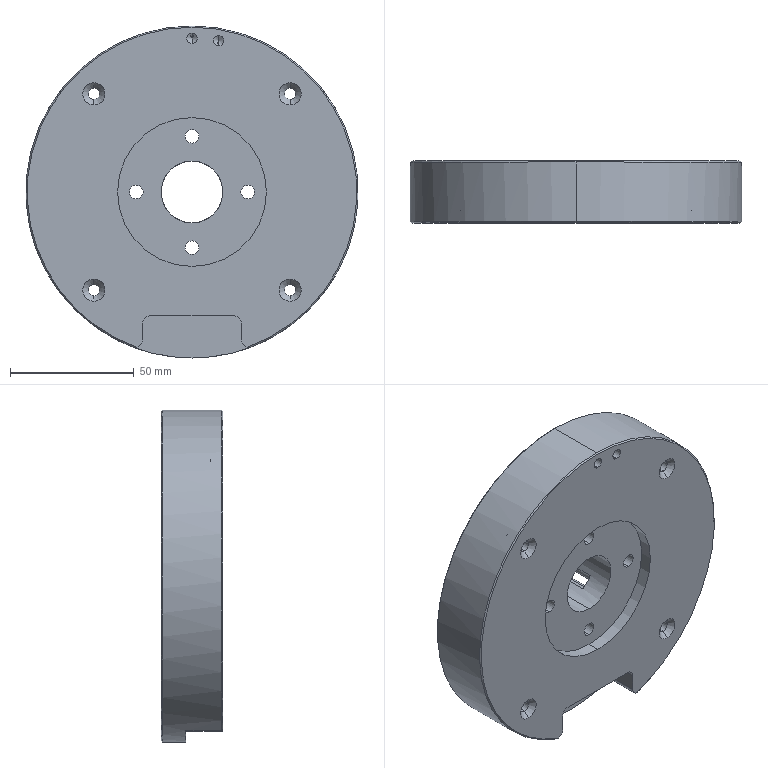Part | SolidWorks | features BaseBody 1 | 1 solid | 138 faces | box 134 x 25 x 134 mm | volume 280686 mm3 | cylinder 74 | cone 34 | plane 30 | commonest cylinder face diameters 21 x12 4 x10 3.3 x8 4.5 x8 5.5 x8 10 x8